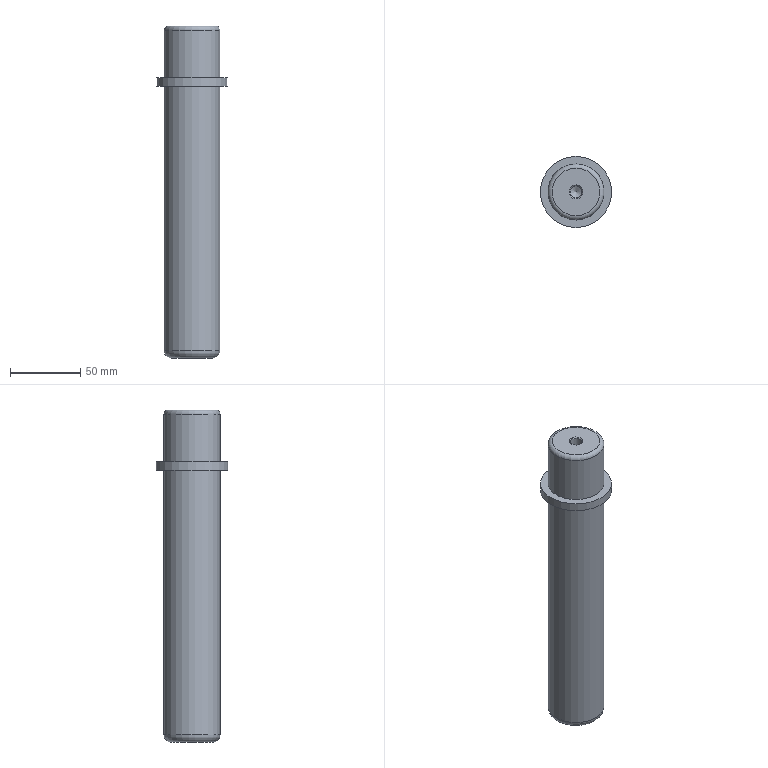Part | STEP file | gslz 2016.10.28-6_id830_x_t | 1 solid | 12 faces | box 50.8 x 50.8 x 237 mm | volume 300382 mm3 | plane 4 | cylinder 4 | torus 2 | cone 2 | commonest cylinder face diameters 40 x2 8.5 x1 50.8 x1
STEP:
#1=CARTESIAN_POINT('',(195.,240.,166.992));
#2=VERTEX_POINT('',#1);
#3=CARTESIAN_POINT('',(195.,245.,166.992));
#4=DIRECTION('',(0.,0.,1.));
#5=DIRECTION('',(0.,-1.,0.));
#6=AXIS2_PLACEMENT_3D('',#3,#4,#5);
#7=CIRCLE('',#6,5.);
#8=EDGE_CURVE('',#2,#2,#7,.T.);
#9=ORIENTED_EDGE('',*,*,#8,.F.);
#10=EDGE_LOOP('',(#9));
#11=FACE_BOUND('',#10,.T.);
#12=CARTESIAN_POINT('',(195.,228.,166.992));
#13=VERTEX_POINT('',#12);
#14=CARTESIAN_POINT('',(195.,245.,166.992));
#15=DIRECTION('',(0.,0.,-1.));
#16=DIRECTION('',(0.,-1.,0.));
#17=AXIS2_PLACEMENT_3D('',#14,#15,#16);
#18=CIRCLE('',#17,17.);
#19=EDGE_CURVE('',#13,#13,#18,.T.);
#20=ORIENTED_EDGE('',*,*,#19,.F.);
#21=EDGE_LOOP('',(#20));
#22=FACE_BOUND('',#21,.T.);
#23=CARTESIAN_POINT('',(195.,245.,166.992));
#24=DIRECTION('',(0.,0.,1.));
#25=DIRECTION('',(0.,1.,0.));
#26=AXIS2_PLACEMENT_3D('',#23,#24,#25);
#27=PLANE('',#26);
#28=ADVANCED_FACE('',(#11,#22),#27,.T.);
#29=CARTESIAN_POINT('',(195.,225.,163.992));
#30=VERTEX_POINT('',#29);
#31=CARTESIAN_POINT('',(195.,245.,163.992));
#32=DIRECTION('',(0.,0.,1.));
#33=DIRECTION('',(0.,-1.,0.));
#34=AXIS2_PLACEMENT_3D('',#31,#32,#33);
#35=CIRCLE('',#34,20.);
#36=EDGE_CURVE('',#30,#30,#35,.T.);
#37=ORIENTED_EDGE('',*,*,#36,.F.);
#38=EDGE_LOOP('',(#37));
#39=FACE_BOUND('',#38,.T.);
#40=CARTESIAN_POINT('',(195.,225.,129.992));
#41=VERTEX_POINT('',#40);
#42=CARTESIAN_POINT('',(195.,245.,129.992));
#43=DIRECTION('',(0.,0.,1.));
#44=DIRECTION('',(0.,-1.,0.));
#45=AXIS2_PLACEMENT_3D('',#42,#43,#44);
#46=CIRCLE('',#45,20.);
#47=EDGE_CURVE('',#41,#41,#46,.T.);
#48=ORIENTED_EDGE('',*,*,#47,.T.);
#49=EDGE_LOOP('',(#48));
#50=FACE_BOUND('',#49,.T.);
#51=CARTESIAN_POINT('',(195.,245.,129.992));
#52=DIRECTION('',(0.,0.,1.));
#53=DIRECTION('',(1.,0.,0.));
#54=AXIS2_PLACEMENT_3D('',#51,#52,#53);
#55=CYLINDRICAL_SURFACE('',#54,20.);
#56=ADVANCED_FACE('',(#39,#50),#55,.T.);
#57=CARTESIAN_POINT('',(195.,270.4,123.992));
#58=VERTEX_POINT('',#57);
#59=CARTESIAN_POINT('',(195.,245.,123.992));
#60=DIRECTION('',(0.,0.,-1.));
#61=DIRECTION('',(0.,1.,0.));
#62=AXIS2_PLACEMENT_3D('',#59,#60,#61);
#63=CIRCLE('',#62,25.4);
#64=EDGE_CURVE('',#58,#58,#63,.T.);
#65=ORIENTED_EDGE('',*,*,#64,.T.);
#66=EDGE_LOOP('',(#65));
#67=FACE_BOUND('',#66,.T.);
#68=CARTESIAN_POINT('',(195.,265.,123.992));
#69=VERTEX_POINT('',#68);
#70=CARTESIAN_POINT('',(195.,245.,123.992));
#71=DIRECTION('',(0.,0.,1.));
#72=DIRECTION('',(0.,1.,0.));
#73=AXIS2_PLACEMENT_3D('',#70,#71,#72);
#74=CIRCLE('',#73,20.);
#75=EDGE_CURVE('',#69,#69,#74,.T.);
#76=ORIENTED_EDGE('',*,*,#75,.T.);
#77=EDGE_LOOP('',(#76));
#78=FACE_BOUND('',#77,.T.);
#79=CARTESIAN_POINT('',(195.,245.,123.992));
#80=DIRECTION('',(0.,0.,-1.));
#81=DIRECTION('',(0.,-1.,0.));
#82=AXIS2_PLACEMENT_3D('',#79,#80,#81);
#83=PLANE('',#82);
#84=ADVANCED_FACE('',(#67,#78),#83,.T.);
#85=ORIENTED_EDGE('',*,*,#47,.F.);
#86=EDGE_LOOP('',(#85));
#87=FACE_BOUND('',#86,.T.);
#88=CARTESIAN_POINT('',(195.,219.6,129.992));
#89=VERTEX_POINT('',#88);
#90=CARTESIAN_POINT('',(195.,245.,129.992));
#91=DIRECTION('',(0.,0.,1.));
#92=DIRECTION('',(0.,-1.,0.));
#93=AXIS2_PLACEMENT_3D('',#90,#91,#92);
#94=CIRCLE('',#93,25.4);
#95=EDGE_CURVE('',#89,#89,#94,.T.);
#96=ORIENTED_EDGE('',*,*,#95,.T.);
#97=EDGE_LOOP('',(#96));
#98=FACE_BOUND('',#97,.T.);
#99=CARTESIAN_POINT('',(195.,245.,129.992));
#100=DIRECTION('',(0.,0.,1.));
#101=DIRECTION('',(0.,1.,0.));
#102=AXIS2_PLACEMENT_3D('',#99,#100,#101);
#103=PLANE('',#102);
#104=ADVANCED_FACE('',(#87,#98),#103,.T.);
#105=ORIENTED_EDGE('',*,*,#64,.F.);
#106=EDGE_LOOP('',(#105));
#107=FACE_BOUND('',#106,.T.);
#108=ORIENTED_EDGE('',*,*,#95,.F.);
#109=EDGE_LOOP('',(#108));
#110=FACE_BOUND('',#109,.T.);
#111=CARTESIAN_POINT('',(195.,245.,129.992));
#112=DIRECTION('',(0.,0.,-1.));
#113=DIRECTION('',(-1.,0.,0.));
#114=AXIS2_PLACEMENT_3D('',#111,#112,#113);
#115=CYLINDRICAL_SURFACE('',#114,25.4);
#116=ADVANCED_FACE('',(#107,#110),#115,.T.);
#117=ORIENTED_EDGE('',*,*,#19,.T.);
#118=EDGE_LOOP('',(#117));
#119=FACE_BOUND('',#118,.T.);
#120=ORIENTED_EDGE('',*,*,#36,.T.);
#121=EDGE_LOOP('',(#120));
#122=FACE_BOUND('',#121,.T.);
#123=CARTESIAN_POINT('',(195.,245.,163.992));
#124=DIRECTION('',(0.,0.,1.));
#125=DIRECTION('',(1.,0.,0.));
#126=AXIS2_PLACEMENT_3D('',#123,#124,#125);
#127=TOROIDAL_SURFACE('',#126,17.,3.);
#128=ADVANCED_FACE('',(#119,#122),#127,.T.);
#129=CARTESIAN_POINT('',(195.,260.,-70.008));
#130=VERTEX_POINT('',#129);
#131=CARTESIAN_POINT('',(195.,245.,-70.008));
#132=DIRECTION('',(0.,0.,1.));
#133=DIRECTION('',(0.,1.,0.));
#134=AXIS2_PLACEMENT_3D('',#131,#132,#133);
#135=CIRCLE('',#134,15.);
#136=EDGE_CURVE('',#130,#130,#135,.T.);
#137=ORIENTED_EDGE('',*,*,#136,.F.);
#138=EDGE_LOOP('',(#137));
#139=FACE_OUTER_BOUND('',#138,.T.);
#140=CARTESIAN_POINT('',(195.,245.,-70.008));
#141=DIRECTION('',(0.,0.,-1.));
#142=DIRECTION('',(-1.,0.,0.));
#143=AXIS2_PLACEMENT_3D('',#140,#141,#142);
#144=PLANE('',#143);
#145=ADVANCED_FACE('',(#139),#144,.T.);
#146=ORIENTED_EDGE('',*,*,#136,.T.);
#147=EDGE_LOOP('',(#146));
#148=FACE_BOUND('',#147,.T.);
#149=CARTESIAN_POINT('',(195.,265.,-65.008));
#150=VERTEX_POINT('',#149);
#151=CARTESIAN_POINT('',(195.,245.,-65.008));
#152=DIRECTION('',(0.,0.,-1.));
#153=DIRECTION('',(0.,1.,0.));
#154=AXIS2_PLACEMENT_3D('',#151,#152,#153);
#155=CIRCLE('',#154,20.);
#156=EDGE_CURVE('',#150,#150,#155,.T.);
#157=ORIENTED_EDGE('',*,*,#156,.T.);
#158=EDGE_LOOP('',(#157));
#159=FACE_BOUND('',#158,.T.);
#160=CARTESIAN_POINT('',(195.,245.,-65.008));
#161=DIRECTION('',(0.,0.,-1.));
#162=DIRECTION('',(0.,-1.,0.));
#163=AXIS2_PLACEMENT_3D('',#160,#161,#162);
#164=TOROIDAL_SURFACE('',#163,15.,5.);
#165=ADVANCED_FACE('',(#148,#159),#164,.T.);
#166=ORIENTED_EDGE('',*,*,#156,.F.);
#167=EDGE_LOOP('',(#166));
#168=FACE_BOUND('',#167,.T.);
#169=ORIENTED_EDGE('',*,*,#75,.F.);
#170=EDGE_LOOP('',(#169));
#171=FACE_BOUND('',#170,.T.);
#172=CARTESIAN_POINT('',(195.,245.,129.992));
#173=DIRECTION('',(0.,0.,-1.));
#174=DIRECTION('',(-1.,0.,0.));
#175=AXIS2_PLACEMENT_3D('',#172,#173,#174);
#176=CYLINDRICAL_SURFACE('',#175,20.);
#177=ADVANCED_FACE('',(#168,#171),#176,.T.);
#178=CARTESIAN_POINT('',(195.,249.25,146.992));
#179=VERTEX_POINT('',#178);
#180=CARTESIAN_POINT('',(195.,245.,146.992));
#181=DIRECTION('',(0.,0.,-1.));
#182=DIRECTION('',(0.,1.,0.));
#183=AXIS2_PLACEMENT_3D('',#180,#181,#182);
#184=CIRCLE('',#183,4.25);
#185=EDGE_CURVE('',#179,#179,#184,.T.);
#186=ORIENTED_EDGE('',*,*,#185,.F.);
#187=EDGE_LOOP('',(#186));
#188=FACE_BOUND('',#187,.T.);
#189=CARTESIAN_POINT('',(195.,245.,144.439));
#190=VERTEX_POINT('',#189);
#191=VERTEX_LOOP('',#190);
#192=FACE_BOUND('',#191,.T.);
#193=CARTESIAN_POINT('',(195.,245.,146.992));
#194=DIRECTION('',(0.,0.,1.));
#195=DIRECTION('',(1.,0.,0.));
#196=AXIS2_PLACEMENT_3D('',#193,#194,#195);
#197=CONICAL_SURFACE('',#196,4.25,59.);
#198=ADVANCED_FACE('',(#188,#192),#197,.F.);
#199=CARTESIAN_POINT('',(195.,240.75,166.242));
#200=VERTEX_POINT('',#199);
#201=CARTESIAN_POINT('',(195.,245.,166.242));
#202=DIRECTION('',(0.,0.,-1.));
#203=DIRECTION('',(0.,-1.,0.));
#204=AXIS2_PLACEMENT_3D('',#201,#202,#203);
#205=CIRCLE('',#204,4.25);
#206=EDGE_CURVE('',#200,#200,#205,.T.);
#207=ORIENTED_EDGE('',*,*,#206,.F.);
#208=EDGE_LOOP('',(#207));
#209=FACE_BOUND('',#208,.T.);
#210=ORIENTED_EDGE('',*,*,#185,.T.);
#211=EDGE_LOOP('',(#210));
#212=FACE_BOUND('',#211,.T.);
#213=CARTESIAN_POINT('',(195.,245.,166.992));
#214=DIRECTION('',(0.,0.,-1.));
#215=DIRECTION('',(-1.,0.,0.));
#216=AXIS2_PLACEMENT_3D('',#213,#214,#215);
#217=CYLINDRICAL_SURFACE('',#216,4.25);
#218=ADVANCED_FACE('',(#209,#212),#217,.F.);
#219=ORIENTED_EDGE('',*,*,#206,.T.);
#220=EDGE_LOOP('',(#219));
#221=FACE_BOUND('',#220,.T.);
#222=ORIENTED_EDGE('',*,*,#8,.T.);
#223=EDGE_LOOP('',(#222));
#224=FACE_BOUND('',#223,.T.);
#225=CARTESIAN_POINT('',(195.,245.,166.992));
#226=DIRECTION('',(0.,0.,1.));
#227=DIRECTION('',(0.,-1.,0.));
#228=AXIS2_PLACEMENT_3D('',#225,#226,#227);
#229=CONICAL_SURFACE('',#228,5.,45.);
#230=ADVANCED_FACE('',(#221,#224),#229,.F.);
#231=CLOSED_SHELL('',(#28,#56,#84,#104,#116,#128,#145,#165,#177,#198,#218,#230));
#232=MANIFOLD_SOLID_BREP('',#231);
#233=(LENGTH_UNIT()NAMED_UNIT(*)SI_UNIT(.MILLI.,.METRE.));
#234=UNCERTAINTY_MEASURE_WITH_UNIT(LENGTH_MEASURE(0.00002),#233,'','');
#235=(NAMED_UNIT(*)PLANE_ANGLE_UNIT()SI_UNIT($,.RADIAN.));
#236=PLANE_ANGLE_MEASURE_WITH_UNIT(PLANE_ANGLE_MEASURE(0.01745),#235);
#237=DIMENSIONAL_EXPONENTS(0.,0.,0.,0.,0.,0.,0.);
#238=(CONVERSION_BASED_UNIT('DEGREE',#236)NAMED_UNIT(#237)PLANE_ANGLE_UNIT());
#239=(NAMED_UNIT(*)SI_UNIT($,.STERADIAN.)SOLID_ANGLE_UNIT());
#240=(GEOMETRIC_REPRESENTATION_CONTEXT(3)GLOBAL_UNCERTAINTY_ASSIGNED_CONTEXT((#234))GLOBAL_UNIT_ASSIGNED_CONTEXT((#233,#238,#239))REPRESENTATION_CONTEXT('',''));
#241=ADVANCED_BREP_SHAPE_REPRESENTATION('',(#232),#240);